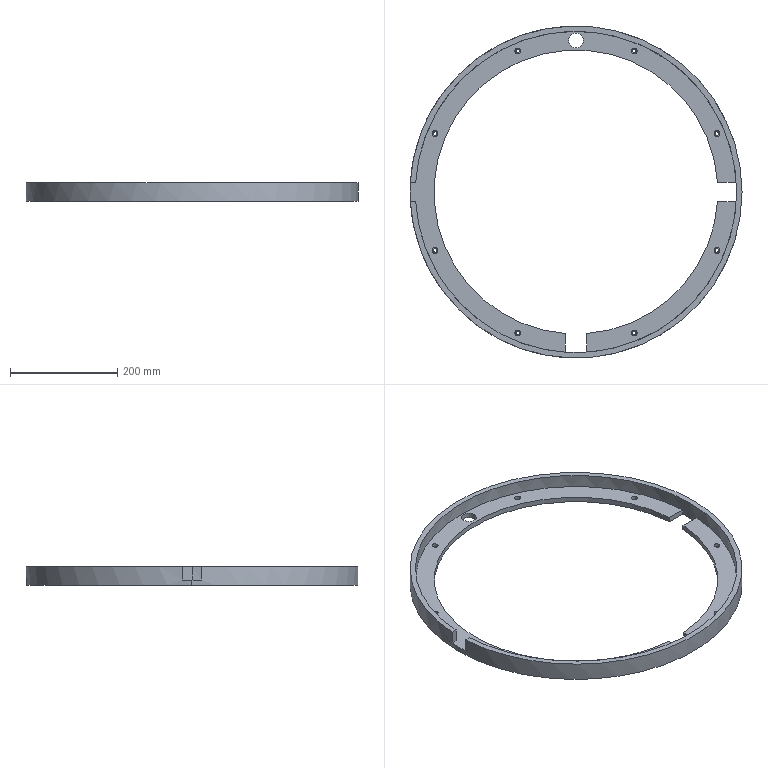Part | STEP file | Stopper bar | 1 solid | 58 faces | box 620 x 620 x 35 mm | volume 1244834 mm3 | cylinder 40 | plane 18 | commonest cylinder face diameters 6.6 x16 11 x16 27 x2 530 x2 600 x2 620 x2